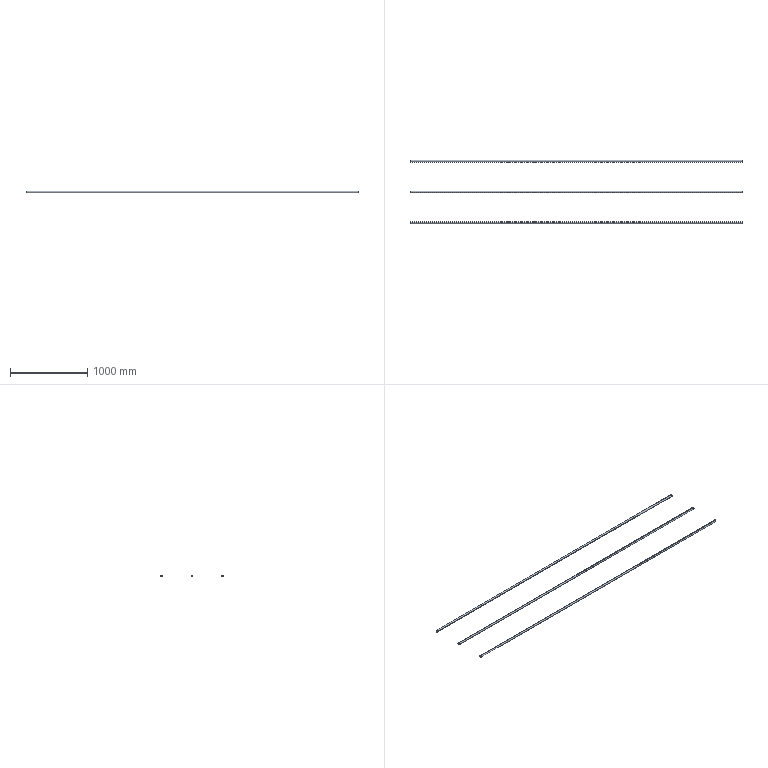Part | STEP file | 电柜护栏4栏杆_Default<As Machined> | 3 solids | 18 faces | box 4293 x 825 x 25 mm | volume 1426235 mm3 | cylinder 12 | plane 6 | commonest cylinder face diameters 22 x6 25 x6
STEP:
#1=CARTESIAN_POINT('',(0.,0.,0.));
#2=DIRECTION('',(0.,0.,1.));
#3=DIRECTION('',(1.,0.,0.));
#4=AXIS2_PLACEMENT_3D('',#1,#2,#3);
#5=CARTESIAN_POINT('',(-4293.,0.,12.5));
#6=VERTEX_POINT('',#5);
#7=CARTESIAN_POINT('',(-4293.,0.,-12.5));
#8=VERTEX_POINT('',#7);
#9=CARTESIAN_POINT('',(-4293.,0.,0.));
#10=DIRECTION('',(-1.,0.,0.));
#11=DIRECTION('',(0.,-1.,0.));
#12=AXIS2_PLACEMENT_3D('',#9,#10,#11);
#13=CIRCLE('',#12,12.5);
#14=CARTESIAN_POINT('',(-4293.,0.,0.));
#15=DIRECTION('',(1.,0.,0.));
#16=DIRECTION('',(0.,0.,-1.));
#17=AXIS2_PLACEMENT_3D('',#14,#15,#16);
#18=CYLINDRICAL_SURFACE('',#17,12.5);
#19=CARTESIAN_POINT('',(4.712,0.));
#20=DIRECTION('',(-1.,0.));
#21=VECTOR('',#20,1.);
#22=LINE('',#19,#21);
#23=(GEOMETRIC_REPRESENTATION_CONTEXT(2)PARAMETRIC_REPRESENTATION_CONTEXT()REPRESENTATION_CONTEXT('',''));
#24=DEFINITIONAL_REPRESENTATION('',(#22),#23);
#25=PCURVE('',#18,#24);
#26=CARTESIAN_POINT('',(-4293.,0.,0.));
#27=DIRECTION('',(-1.,0.,0.));
#28=DIRECTION('',(0.,-1.,0.));
#29=AXIS2_PLACEMENT_3D('',#26,#27,#28);
#30=PLANE('',#29);
#31=CARTESIAN_POINT('',(0.,0.));
#32=DIRECTION('',(1.,0.));
#33=AXIS2_PLACEMENT_2D('',#31,#32);
#34=CIRCLE('',#33,12.5);
#35=(GEOMETRIC_REPRESENTATION_CONTEXT(2)PARAMETRIC_REPRESENTATION_CONTEXT()REPRESENTATION_CONTEXT('',''));
#36=DEFINITIONAL_REPRESENTATION('',(#34),#35);
#37=PCURVE('',#30,#36);
#38=SURFACE_CURVE('',#13,(#25,#37),.PCURVE_S1.);
#39=EDGE_CURVE('',#6,#8,#38,.T.);
#40=ORIENTED_EDGE('',*,*,#39,.F.);
#41=CARTESIAN_POINT('',(0.,0.,12.5));
#42=VERTEX_POINT('',#41);
#43=CARTESIAN_POINT('',(-4293.,0.,12.5));
#44=DIRECTION('',(1.,0.,0.));
#45=VECTOR('',#44,1.);
#46=LINE('',#43,#45);
#47=CARTESIAN_POINT('',(3.142,0.));
#48=DIRECTION('',(0.,1.));
#49=VECTOR('',#48,1.);
#50=LINE('',#47,#49);
#51=(GEOMETRIC_REPRESENTATION_CONTEXT(2)PARAMETRIC_REPRESENTATION_CONTEXT()REPRESENTATION_CONTEXT('',''));
#52=DEFINITIONAL_REPRESENTATION('',(#50),#51);
#53=PCURVE('',#18,#52);
#54=CARTESIAN_POINT('',(-4293.,0.,0.));
#55=DIRECTION('',(1.,0.,0.));
#56=DIRECTION('',(0.,0.,-1.));
#57=AXIS2_PLACEMENT_3D('',#54,#55,#56);
#58=CYLINDRICAL_SURFACE('',#57,12.5);
#59=CARTESIAN_POINT('',(3.142,0.));
#60=DIRECTION('',(0.,1.));
#61=VECTOR('',#60,1.);
#62=LINE('',#59,#61);
#63=(GEOMETRIC_REPRESENTATION_CONTEXT(2)PARAMETRIC_REPRESENTATION_CONTEXT()REPRESENTATION_CONTEXT('',''));
#64=DEFINITIONAL_REPRESENTATION('',(#62),#63);
#65=PCURVE('',#58,#64);
#66=SURFACE_CURVE('',#46,(#53,#65),.PCURVE_S1.);
#67=EDGE_CURVE('',#6,#42,#66,.T.);
#68=ORIENTED_EDGE('',*,*,#67,.T.);
#69=CARTESIAN_POINT('',(0.,0.,-12.5));
#70=VERTEX_POINT('',#69);
#71=CARTESIAN_POINT('',(0.,0.,0.));
#72=DIRECTION('',(-1.,0.,0.));
#73=DIRECTION('',(0.,-1.,0.));
#74=AXIS2_PLACEMENT_3D('',#71,#72,#73);
#75=CIRCLE('',#74,12.5);
#76=CARTESIAN_POINT('',(4.712,4293.));
#77=DIRECTION('',(-1.,0.));
#78=VECTOR('',#77,1.);
#79=LINE('',#76,#78);
#80=(GEOMETRIC_REPRESENTATION_CONTEXT(2)PARAMETRIC_REPRESENTATION_CONTEXT()REPRESENTATION_CONTEXT('',''));
#81=DEFINITIONAL_REPRESENTATION('',(#79),#80);
#82=PCURVE('',#18,#81);
#83=CARTESIAN_POINT('',(0.,0.,0.));
#84=DIRECTION('',(-1.,0.,0.));
#85=DIRECTION('',(0.,-1.,0.));
#86=AXIS2_PLACEMENT_3D('',#83,#84,#85);
#87=PLANE('',#86);
#88=CARTESIAN_POINT('',(0.,0.));
#89=DIRECTION('',(1.,0.));
#90=AXIS2_PLACEMENT_2D('',#88,#89);
#91=CIRCLE('',#90,12.5);
#92=(GEOMETRIC_REPRESENTATION_CONTEXT(2)PARAMETRIC_REPRESENTATION_CONTEXT()REPRESENTATION_CONTEXT('',''));
#93=DEFINITIONAL_REPRESENTATION('',(#91),#92);
#94=PCURVE('',#87,#93);
#95=SURFACE_CURVE('',#75,(#82,#94),.PCURVE_S1.);
#96=EDGE_CURVE('',#42,#70,#95,.T.);
#97=ORIENTED_EDGE('',*,*,#96,.T.);
#98=CARTESIAN_POINT('',(-4293.,0.,-12.5));
#99=DIRECTION('',(1.,0.,0.));
#100=VECTOR('',#99,1.);
#101=LINE('',#98,#100);
#102=CARTESIAN_POINT('',(0.,0.));
#103=DIRECTION('',(0.,1.));
#104=VECTOR('',#103,1.);
#105=LINE('',#102,#104);
#106=(GEOMETRIC_REPRESENTATION_CONTEXT(2)PARAMETRIC_REPRESENTATION_CONTEXT()REPRESENTATION_CONTEXT('',''));
#107=DEFINITIONAL_REPRESENTATION('',(#105),#106);
#108=PCURVE('',#18,#107);
#109=CARTESIAN_POINT('',(6.283,0.));
#110=DIRECTION('',(0.,1.));
#111=VECTOR('',#110,1.);
#112=LINE('',#109,#111);
#113=(GEOMETRIC_REPRESENTATION_CONTEXT(2)PARAMETRIC_REPRESENTATION_CONTEXT()REPRESENTATION_CONTEXT('',''));
#114=DEFINITIONAL_REPRESENTATION('',(#112),#113);
#115=PCURVE('',#58,#114);
#116=SURFACE_CURVE('',#101,(#108,#115),.PCURVE_S1.);
#117=EDGE_CURVE('',#8,#70,#116,.T.);
#118=ORIENTED_EDGE('',*,*,#117,.F.);
#119=EDGE_LOOP('',(#40,#68,#97,#118));
#120=FACE_BOUND('',#119,.T.);
#121=ADVANCED_FACE('',(#120),#18,.T.);
#122=CARTESIAN_POINT('',(-4293.,0.,-11.));
#123=VERTEX_POINT('',#122);
#124=CARTESIAN_POINT('',(0.,0.,-11.));
#125=VERTEX_POINT('',#124);
#126=CARTESIAN_POINT('',(-4293.,0.,-11.));
#127=DIRECTION('',(1.,0.,0.));
#128=VECTOR('',#127,1.);
#129=LINE('',#126,#128);
#130=CARTESIAN_POINT('',(-4293.,0.,0.));
#131=DIRECTION('',(1.,0.,0.));
#132=DIRECTION('',(0.,0.,-1.));
#133=AXIS2_PLACEMENT_3D('',#130,#131,#132);
#134=CYLINDRICAL_SURFACE('',#133,11.);
#135=CARTESIAN_POINT('',(6.283,0.));
#136=DIRECTION('',(0.,1.));
#137=VECTOR('',#136,1.);
#138=LINE('',#135,#137);
#139=(GEOMETRIC_REPRESENTATION_CONTEXT(2)PARAMETRIC_REPRESENTATION_CONTEXT()REPRESENTATION_CONTEXT('',''));
#140=DEFINITIONAL_REPRESENTATION('',(#138),#139);
#141=PCURVE('',#134,#140);
#142=CARTESIAN_POINT('',(-4293.,0.,0.));
#143=DIRECTION('',(1.,0.,0.));
#144=DIRECTION('',(0.,0.,-1.));
#145=AXIS2_PLACEMENT_3D('',#142,#143,#144);
#146=CYLINDRICAL_SURFACE('',#145,11.);
#147=CARTESIAN_POINT('',(0.,0.));
#148=DIRECTION('',(0.,1.));
#149=VECTOR('',#148,1.);
#150=LINE('',#147,#149);
#151=(GEOMETRIC_REPRESENTATION_CONTEXT(2)PARAMETRIC_REPRESENTATION_CONTEXT()REPRESENTATION_CONTEXT('',''));
#152=DEFINITIONAL_REPRESENTATION('',(#150),#151);
#153=PCURVE('',#146,#152);
#154=SURFACE_CURVE('',#129,(#141,#153),.PCURVE_S1.);
#155=EDGE_CURVE('',#123,#125,#154,.T.);
#156=ORIENTED_EDGE('',*,*,#155,.T.);
#157=CARTESIAN_POINT('',(0.,0.,11.));
#158=VERTEX_POINT('',#157);
#159=CARTESIAN_POINT('',(0.,0.,0.));
#160=DIRECTION('',(-1.,0.,0.));
#161=DIRECTION('',(0.,-1.,0.));
#162=AXIS2_PLACEMENT_3D('',#159,#160,#161);
#163=CIRCLE('',#162,11.);
#164=CARTESIAN_POINT('',(10.996,4293.));
#165=DIRECTION('',(-1.,0.));
#166=VECTOR('',#165,1.);
#167=LINE('',#164,#166);
#168=(GEOMETRIC_REPRESENTATION_CONTEXT(2)PARAMETRIC_REPRESENTATION_CONTEXT()REPRESENTATION_CONTEXT('',''));
#169=DEFINITIONAL_REPRESENTATION('',(#167),#168);
#170=PCURVE('',#134,#169);
#171=CARTESIAN_POINT('',(0.,0.));
#172=DIRECTION('',(1.,0.));
#173=AXIS2_PLACEMENT_2D('',#171,#172);
#174=CIRCLE('',#173,11.);
#175=(GEOMETRIC_REPRESENTATION_CONTEXT(2)PARAMETRIC_REPRESENTATION_CONTEXT()REPRESENTATION_CONTEXT('',''));
#176=DEFINITIONAL_REPRESENTATION('',(#174),#175);
#177=PCURVE('',#87,#176);
#178=SURFACE_CURVE('',#163,(#170,#177),.PCURVE_S1.);
#179=EDGE_CURVE('',#125,#158,#178,.T.);
#180=ORIENTED_EDGE('',*,*,#179,.T.);
#181=CARTESIAN_POINT('',(-4293.,0.,11.));
#182=VERTEX_POINT('',#181);
#183=CARTESIAN_POINT('',(-4293.,0.,11.));
#184=DIRECTION('',(1.,0.,0.));
#185=VECTOR('',#184,1.);
#186=LINE('',#183,#185);
#187=CARTESIAN_POINT('',(3.142,0.));
#188=DIRECTION('',(0.,1.));
#189=VECTOR('',#188,1.);
#190=LINE('',#187,#189);
#191=(GEOMETRIC_REPRESENTATION_CONTEXT(2)PARAMETRIC_REPRESENTATION_CONTEXT()REPRESENTATION_CONTEXT('',''));
#192=DEFINITIONAL_REPRESENTATION('',(#190),#191);
#193=PCURVE('',#134,#192);
#194=CARTESIAN_POINT('',(3.142,0.));
#195=DIRECTION('',(0.,1.));
#196=VECTOR('',#195,1.);
#197=LINE('',#194,#196);
#198=(GEOMETRIC_REPRESENTATION_CONTEXT(2)PARAMETRIC_REPRESENTATION_CONTEXT()REPRESENTATION_CONTEXT('',''));
#199=DEFINITIONAL_REPRESENTATION('',(#197),#198);
#200=PCURVE('',#146,#199);
#201=SURFACE_CURVE('',#186,(#193,#200),.PCURVE_S1.);
#202=EDGE_CURVE('',#182,#158,#201,.T.);
#203=ORIENTED_EDGE('',*,*,#202,.F.);
#204=CARTESIAN_POINT('',(-4293.,0.,0.));
#205=DIRECTION('',(-1.,0.,0.));
#206=DIRECTION('',(0.,-1.,0.));
#207=AXIS2_PLACEMENT_3D('',#204,#205,#206);
#208=CIRCLE('',#207,11.);
#209=CARTESIAN_POINT('',(10.996,0.));
#210=DIRECTION('',(-1.,0.));
#211=VECTOR('',#210,1.);
#212=LINE('',#209,#211);
#213=(GEOMETRIC_REPRESENTATION_CONTEXT(2)PARAMETRIC_REPRESENTATION_CONTEXT()REPRESENTATION_CONTEXT('',''));
#214=DEFINITIONAL_REPRESENTATION('',(#212),#213);
#215=PCURVE('',#134,#214);
#216=CARTESIAN_POINT('',(0.,0.));
#217=DIRECTION('',(1.,0.));
#218=AXIS2_PLACEMENT_2D('',#216,#217);
#219=CIRCLE('',#218,11.);
#220=(GEOMETRIC_REPRESENTATION_CONTEXT(2)PARAMETRIC_REPRESENTATION_CONTEXT()REPRESENTATION_CONTEXT('',''));
#221=DEFINITIONAL_REPRESENTATION('',(#219),#220);
#222=PCURVE('',#30,#221);
#223=SURFACE_CURVE('',#208,(#215,#222),.PCURVE_S1.);
#224=EDGE_CURVE('',#123,#182,#223,.T.);
#225=ORIENTED_EDGE('',*,*,#224,.F.);
#226=EDGE_LOOP('',(#156,#180,#203,#225));
#227=FACE_BOUND('',#226,.F.);
#228=ADVANCED_FACE('',(#227),#134,.F.);
#229=CARTESIAN_POINT('',(0.,0.,0.));
#230=DIRECTION('',(-1.,0.,0.));
#231=DIRECTION('',(0.,-1.,0.));
#232=AXIS2_PLACEMENT_3D('',#229,#230,#231);
#233=CIRCLE('',#232,11.);
#234=CARTESIAN_POINT('',(4.712,4293.));
#235=DIRECTION('',(-1.,0.));
#236=VECTOR('',#235,1.);
#237=LINE('',#234,#236);
#238=(GEOMETRIC_REPRESENTATION_CONTEXT(2)PARAMETRIC_REPRESENTATION_CONTEXT()REPRESENTATION_CONTEXT('',''));
#239=DEFINITIONAL_REPRESENTATION('',(#237),#238);
#240=PCURVE('',#146,#239);
#241=CARTESIAN_POINT('',(0.,0.));
#242=DIRECTION('',(1.,0.));
#243=AXIS2_PLACEMENT_2D('',#241,#242);
#244=CIRCLE('',#243,11.);
#245=(GEOMETRIC_REPRESENTATION_CONTEXT(2)PARAMETRIC_REPRESENTATION_CONTEXT()REPRESENTATION_CONTEXT('',''));
#246=DEFINITIONAL_REPRESENTATION('',(#244),#245);
#247=PCURVE('',#87,#246);
#248=SURFACE_CURVE('',#233,(#240,#247),.PCURVE_S1.);
#249=EDGE_CURVE('',#158,#125,#248,.T.);
#250=ORIENTED_EDGE('',*,*,#249,.T.);
#251=ORIENTED_EDGE('',*,*,#155,.F.);
#252=CARTESIAN_POINT('',(-4293.,0.,0.));
#253=DIRECTION('',(-1.,0.,0.));
#254=DIRECTION('',(0.,-1.,0.));
#255=AXIS2_PLACEMENT_3D('',#252,#253,#254);
#256=CIRCLE('',#255,11.);
#257=CARTESIAN_POINT('',(4.712,0.));
#258=DIRECTION('',(-1.,0.));
#259=VECTOR('',#258,1.);
#260=LINE('',#257,#259);
#261=(GEOMETRIC_REPRESENTATION_CONTEXT(2)PARAMETRIC_REPRESENTATION_CONTEXT()REPRESENTATION_CONTEXT('',''));
#262=DEFINITIONAL_REPRESENTATION('',(#260),#261);
#263=PCURVE('',#146,#262);
#264=CARTESIAN_POINT('',(0.,0.));
#265=DIRECTION('',(1.,0.));
#266=AXIS2_PLACEMENT_2D('',#264,#265);
#267=CIRCLE('',#266,11.);
#268=(GEOMETRIC_REPRESENTATION_CONTEXT(2)PARAMETRIC_REPRESENTATION_CONTEXT()REPRESENTATION_CONTEXT('',''));
#269=DEFINITIONAL_REPRESENTATION('',(#267),#268);
#270=PCURVE('',#30,#269);
#271=SURFACE_CURVE('',#256,(#263,#270),.PCURVE_S1.);
#272=EDGE_CURVE('',#182,#123,#271,.T.);
#273=ORIENTED_EDGE('',*,*,#272,.F.);
#274=ORIENTED_EDGE('',*,*,#202,.T.);
#275=EDGE_LOOP('',(#250,#251,#273,#274));
#276=FACE_BOUND('',#275,.F.);
#277=ADVANCED_FACE('',(#276),#146,.F.);
#278=ORIENTED_EDGE('',*,*,#67,.F.);
#279=CARTESIAN_POINT('',(-4293.,0.,0.));
#280=DIRECTION('',(-1.,0.,0.));
#281=DIRECTION('',(0.,-1.,0.));
#282=AXIS2_PLACEMENT_3D('',#279,#280,#281);
#283=CIRCLE('',#282,12.5);
#284=CARTESIAN_POINT('',(10.996,0.));
#285=DIRECTION('',(-1.,0.));
#286=VECTOR('',#285,1.);
#287=LINE('',#284,#286);
#288=(GEOMETRIC_REPRESENTATION_CONTEXT(2)PARAMETRIC_REPRESENTATION_CONTEXT()REPRESENTATION_CONTEXT('',''));
#289=DEFINITIONAL_REPRESENTATION('',(#287),#288);
#290=PCURVE('',#58,#289);
#291=CARTESIAN_POINT('',(0.,0.));
#292=DIRECTION('',(1.,0.));
#293=AXIS2_PLACEMENT_2D('',#291,#292);
#294=CIRCLE('',#293,12.5);
#295=(GEOMETRIC_REPRESENTATION_CONTEXT(2)PARAMETRIC_REPRESENTATION_CONTEXT()REPRESENTATION_CONTEXT('',''));
#296=DEFINITIONAL_REPRESENTATION('',(#294),#295);
#297=PCURVE('',#30,#296);
#298=SURFACE_CURVE('',#283,(#290,#297),.PCURVE_S1.);
#299=EDGE_CURVE('',#8,#6,#298,.T.);
#300=ORIENTED_EDGE('',*,*,#299,.F.);
#301=ORIENTED_EDGE('',*,*,#117,.T.);
#302=CARTESIAN_POINT('',(0.,0.,0.));
#303=DIRECTION('',(-1.,0.,0.));
#304=DIRECTION('',(0.,-1.,0.));
#305=AXIS2_PLACEMENT_3D('',#302,#303,#304);
#306=CIRCLE('',#305,12.5);
#307=CARTESIAN_POINT('',(10.996,4293.));
#308=DIRECTION('',(-1.,0.));
#309=VECTOR('',#308,1.);
#310=LINE('',#307,#309);
#311=(GEOMETRIC_REPRESENTATION_CONTEXT(2)PARAMETRIC_REPRESENTATION_CONTEXT()REPRESENTATION_CONTEXT('',''));
#312=DEFINITIONAL_REPRESENTATION('',(#310),#311);
#313=PCURVE('',#58,#312);
#314=CARTESIAN_POINT('',(0.,0.));
#315=DIRECTION('',(1.,0.));
#316=AXIS2_PLACEMENT_2D('',#314,#315);
#317=CIRCLE('',#316,12.5);
#318=(GEOMETRIC_REPRESENTATION_CONTEXT(2)PARAMETRIC_REPRESENTATION_CONTEXT()REPRESENTATION_CONTEXT('',''));
#319=DEFINITIONAL_REPRESENTATION('',(#317),#318);
#320=PCURVE('',#87,#319);
#321=SURFACE_CURVE('',#306,(#313,#320),.PCURVE_S1.);
#322=EDGE_CURVE('',#70,#42,#321,.T.);
#323=ORIENTED_EDGE('',*,*,#322,.T.);
#324=EDGE_LOOP('',(#278,#300,#301,#323));
#325=FACE_BOUND('',#324,.T.);
#326=ADVANCED_FACE('',(#325),#58,.T.);
#327=ORIENTED_EDGE('',*,*,#224,.F.);
#328=ORIENTED_EDGE('',*,*,#272,.F.);
#329=EDGE_LOOP('',(#327,#328));
#330=FACE_BOUND('',#329,.T.);
#331=ORIENTED_EDGE('',*,*,#299,.T.);
#332=ORIENTED_EDGE('',*,*,#39,.T.);
#333=EDGE_LOOP('',(#331,#332));
#334=FACE_BOUND('',#333,.T.);
#335=ADVANCED_FACE('',(#330,#334),#30,.T.);
#336=ORIENTED_EDGE('',*,*,#179,.T.);
#337=ORIENTED_EDGE('',*,*,#249,.T.);
#338=EDGE_LOOP('',(#336,#337));
#339=FACE_BOUND('',#338,.T.);
#340=ORIENTED_EDGE('',*,*,#322,.F.);
#341=ORIENTED_EDGE('',*,*,#96,.F.);
#342=EDGE_LOOP('',(#340,#341));
#343=FACE_BOUND('',#342,.T.);
#344=ADVANCED_FACE('',(#339,#343),#87,.F.);
#345=CLOSED_SHELL('',(#121,#228,#277,#326,#335,#344));
#346=MANIFOLD_SOLID_BREP('',#345);
#347=CARTESIAN_POINT('',(-4293.,787.5,0.));
#348=VERTEX_POINT('',#347);
#349=CARTESIAN_POINT('',(-4293.,812.5,0.));
#350=VERTEX_POINT('',#349);
#351=CARTESIAN_POINT('',(-4293.,800.,0.));
#352=DIRECTION('',(-1.,0.,0.));
#353=DIRECTION('',(0.,-1.,0.));
#354=AXIS2_PLACEMENT_3D('',#351,#352,#353);
#355=CIRCLE('',#354,12.5);
#356=CARTESIAN_POINT('',(-4293.,800.,0.));
#357=DIRECTION('',(1.,0.,0.));
#358=DIRECTION('',(0.,1.,0.));
#359=AXIS2_PLACEMENT_3D('',#356,#357,#358);
#360=CYLINDRICAL_SURFACE('',#359,12.5);
#361=CARTESIAN_POINT('',(3.142,0.));
#362=DIRECTION('',(-1.,0.));
#363=VECTOR('',#362,1.);
#364=LINE('',#361,#363);
#365=(GEOMETRIC_REPRESENTATION_CONTEXT(2)PARAMETRIC_REPRESENTATION_CONTEXT()REPRESENTATION_CONTEXT('',''));
#366=DEFINITIONAL_REPRESENTATION('',(#364),#365);
#367=PCURVE('',#360,#366);
#368=CARTESIAN_POINT('',(-4293.,800.,0.));
#369=DIRECTION('',(-1.,0.,0.));
#370=DIRECTION('',(0.,-1.,0.));
#371=AXIS2_PLACEMENT_3D('',#368,#369,#370);
#372=PLANE('',#371);
#373=CARTESIAN_POINT('',(0.,0.));
#374=DIRECTION('',(1.,0.));
#375=AXIS2_PLACEMENT_2D('',#373,#374);
#376=CIRCLE('',#375,12.5);
#377=(GEOMETRIC_REPRESENTATION_CONTEXT(2)PARAMETRIC_REPRESENTATION_CONTEXT()REPRESENTATION_CONTEXT('',''));
#378=DEFINITIONAL_REPRESENTATION('',(#376),#377);
#379=PCURVE('',#372,#378);
#380=SURFACE_CURVE('',#355,(#367,#379),.PCURVE_S1.);
#381=EDGE_CURVE('',#348,#350,#380,.T.);
#382=ORIENTED_EDGE('',*,*,#381,.F.);
#383=CARTESIAN_POINT('',(0.,787.5,0.));
#384=VERTEX_POINT('',#383);
#385=CARTESIAN_POINT('',(-4293.,787.5,0.));
#386=DIRECTION('',(1.,0.,0.));
#387=VECTOR('',#386,1.);
#388=LINE('',#385,#387);
#389=CARTESIAN_POINT('',(3.142,0.));
#390=DIRECTION('',(0.,1.));
#391=VECTOR('',#390,1.);
#392=LINE('',#389,#391);
#393=(GEOMETRIC_REPRESENTATION_CONTEXT(2)PARAMETRIC_REPRESENTATION_CONTEXT()REPRESENTATION_CONTEXT('',''));
#394=DEFINITIONAL_REPRESENTATION('',(#392),#393);
#395=PCURVE('',#360,#394);
#396=CARTESIAN_POINT('',(-4293.,800.,0.));
#397=DIRECTION('',(1.,0.,0.));
#398=DIRECTION('',(0.,1.,0.));
#399=AXIS2_PLACEMENT_3D('',#396,#397,#398);
#400=CYLINDRICAL_SURFACE('',#399,12.5);
#401=CARTESIAN_POINT('',(3.142,0.));
#402=DIRECTION('',(0.,1.));
#403=VECTOR('',#402,1.);
#404=LINE('',#401,#403);
#405=(GEOMETRIC_REPRESENTATION_CONTEXT(2)PARAMETRIC_REPRESENTATION_CONTEXT()REPRESENTATION_CONTEXT('',''));
#406=DEFINITIONAL_REPRESENTATION('',(#404),#405);
#407=PCURVE('',#400,#406);
#408=SURFACE_CURVE('',#388,(#395,#407),.PCURVE_S1.);
#409=EDGE_CURVE('',#348,#384,#408,.T.);
#410=ORIENTED_EDGE('',*,*,#409,.T.);
#411=CARTESIAN_POINT('',(0.,812.5,0.));
#412=VERTEX_POINT('',#411);
#413=CARTESIAN_POINT('',(0.,800.,0.));
#414=DIRECTION('',(-1.,0.,0.));
#415=DIRECTION('',(0.,-1.,0.));
#416=AXIS2_PLACEMENT_3D('',#413,#414,#415);
#417=CIRCLE('',#416,12.5);
#418=CARTESIAN_POINT('',(3.142,4293.));
#419=DIRECTION('',(-1.,0.));
#420=VECTOR('',#419,1.);
#421=LINE('',#418,#420);
#422=(GEOMETRIC_REPRESENTATION_CONTEXT(2)PARAMETRIC_REPRESENTATION_CONTEXT()REPRESENTATION_CONTEXT('',''));
#423=DEFINITIONAL_REPRESENTATION('',(#421),#422);
#424=PCURVE('',#360,#423);
#425=CARTESIAN_POINT('',(0.,800.,0.));
#426=DIRECTION('',(-1.,0.,0.));
#427=DIRECTION('',(0.,-1.,0.));
#428=AXIS2_PLACEMENT_3D('',#425,#426,#427);
#429=PLANE('',#428);
#430=CARTESIAN_POINT('',(0.,0.));
#431=DIRECTION('',(1.,0.));
#432=AXIS2_PLACEMENT_2D('',#430,#431);
#433=CIRCLE('',#432,12.5);
#434=(GEOMETRIC_REPRESENTATION_CONTEXT(2)PARAMETRIC_REPRESENTATION_CONTEXT()REPRESENTATION_CONTEXT('',''));
#435=DEFINITIONAL_REPRESENTATION('',(#433),#434);
#436=PCURVE('',#429,#435);
#437=SURFACE_CURVE('',#417,(#424,#436),.PCURVE_S1.);
#438=EDGE_CURVE('',#384,#412,#437,.T.);
#439=ORIENTED_EDGE('',*,*,#438,.T.);
#440=CARTESIAN_POINT('',(-4293.,812.5,0.));
#441=DIRECTION('',(1.,0.,0.));
#442=VECTOR('',#441,1.);
#443=LINE('',#440,#442);
#444=CARTESIAN_POINT('',(0.,0.));
#445=DIRECTION('',(0.,1.));
#446=VECTOR('',#445,1.);
#447=LINE('',#444,#446);
#448=(GEOMETRIC_REPRESENTATION_CONTEXT(2)PARAMETRIC_REPRESENTATION_CONTEXT()REPRESENTATION_CONTEXT('',''));
#449=DEFINITIONAL_REPRESENTATION('',(#447),#448);
#450=PCURVE('',#360,#449);
#451=CARTESIAN_POINT('',(6.283,0.));
#452=DIRECTION('',(0.,1.));
#453=VECTOR('',#452,1.);
#454=LINE('',#451,#453);
#455=(GEOMETRIC_REPRESENTATION_CONTEXT(2)PARAMETRIC_REPRESENTATION_CONTEXT()REPRESENTATION_CONTEXT('',''));
#456=DEFINITIONAL_REPRESENTATION('',(#454),#455);
#457=PCURVE('',#400,#456);
#458=SURFACE_CURVE('',#443,(#450,#457),.PCURVE_S1.);
#459=EDGE_CURVE('',#350,#412,#458,.T.);
#460=ORIENTED_EDGE('',*,*,#459,.F.);
#461=EDGE_LOOP('',(#382,#410,#439,#460));
#462=FACE_BOUND('',#461,.T.);
#463=ADVANCED_FACE('',(#462),#360,.T.);
#464=CARTESIAN_POINT('',(-4293.,811.,0.));
#465=VERTEX_POINT('',#464);
#466=CARTESIAN_POINT('',(0.,811.,0.));
#467=VERTEX_POINT('',#466);
#468=CARTESIAN_POINT('',(-4293.,811.,0.));
#469=DIRECTION('',(1.,0.,0.));
#470=VECTOR('',#469,1.);
#471=LINE('',#468,#470);
#472=CARTESIAN_POINT('',(-4293.,800.,0.));
#473=DIRECTION('',(1.,0.,0.));
#474=DIRECTION('',(0.,1.,0.));
#475=AXIS2_PLACEMENT_3D('',#472,#473,#474);
#476=CYLINDRICAL_SURFACE('',#475,11.);
#477=CARTESIAN_POINT('',(6.283,0.));
#478=DIRECTION('',(0.,1.));
#479=VECTOR('',#478,1.);
#480=LINE('',#477,#479);
#481=(GEOMETRIC_REPRESENTATION_CONTEXT(2)PARAMETRIC_REPRESENTATION_CONTEXT()REPRESENTATION_CONTEXT('',''));
#482=DEFINITIONAL_REPRESENTATION('',(#480),#481);
#483=PCURVE('',#476,#482);
#484=CARTESIAN_POINT('',(-4293.,800.,0.));
#485=DIRECTION('',(1.,0.,0.));
#486=DIRECTION('',(0.,1.,0.));
#487=AXIS2_PLACEMENT_3D('',#484,#485,#486);
#488=CYLINDRICAL_SURFACE('',#487,11.);
#489=CARTESIAN_POINT('',(0.,0.));
#490=DIRECTION('',(0.,1.));
#491=VECTOR('',#490,1.);
#492=LINE('',#489,#491);
#493=(GEOMETRIC_REPRESENTATION_CONTEXT(2)PARAMETRIC_REPRESENTATION_CONTEXT()REPRESENTATION_CONTEXT('',''));
#494=DEFINITIONAL_REPRESENTATION('',(#492),#493);
#495=PCURVE('',#488,#494);
#496=SURFACE_CURVE('',#471,(#483,#495),.PCURVE_S1.);
#497=EDGE_CURVE('',#465,#467,#496,.T.);
#498=ORIENTED_EDGE('',*,*,#497,.T.);
#499=CARTESIAN_POINT('',(0.,789.,0.));
#500=VERTEX_POINT('',#499);
#501=CARTESIAN_POINT('',(0.,800.,0.));
#502=DIRECTION('',(-1.,0.,0.));
#503=DIRECTION('',(0.,-1.,0.));
#504=AXIS2_PLACEMENT_3D('',#501,#502,#503);
#505=CIRCLE('',#504,11.);
#506=CARTESIAN_POINT('',(9.425,4293.));
#507=DIRECTION('',(-1.,0.));
#508=VECTOR('',#507,1.);
#509=LINE('',#506,#508);
#510=(GEOMETRIC_REPRESENTATION_CONTEXT(2)PARAMETRIC_REPRESENTATION_CONTEXT()REPRESENTATION_CONTEXT('',''));
#511=DEFINITIONAL_REPRESENTATION('',(#509),#510);
#512=PCURVE('',#476,#511);
#513=CARTESIAN_POINT('',(0.,0.));
#514=DIRECTION('',(1.,0.));
#515=AXIS2_PLACEMENT_2D('',#513,#514);
#516=CIRCLE('',#515,11.);
#517=(GEOMETRIC_REPRESENTATION_CONTEXT(2)PARAMETRIC_REPRESENTATION_CONTEXT()REPRESENTATION_CONTEXT('',''));
#518=DEFINITIONAL_REPRESENTATION('',(#516),#517);
#519=PCURVE('',#429,#518);
#520=SURFACE_CURVE('',#505,(#512,#519),.PCURVE_S1.);
#521=EDGE_CURVE('',#467,#500,#520,.T.);
#522=ORIENTED_EDGE('',*,*,#521,.T.);
#523=CARTESIAN_POINT('',(-4293.,789.,0.));
#524=VERTEX_POINT('',#523);
#525=CARTESIAN_POINT('',(-4293.,789.,0.));
#526=DIRECTION('',(1.,0.,0.));
#527=VECTOR('',#526,1.);
#528=LINE('',#525,#527);
#529=CARTESIAN_POINT('',(3.142,0.));
#530=DIRECTION('',(0.,1.));
#531=VECTOR('',#530,1.);
#532=LINE('',#529,#531);
#533=(GEOMETRIC_REPRESENTATION_CONTEXT(2)PARAMETRIC_REPRESENTATION_CONTEXT()REPRESENTATION_CONTEXT('',''));
#534=DEFINITIONAL_REPRESENTATION('',(#532),#533);
#535=PCURVE('',#476,#534);
#536=CARTESIAN_POINT('',(3.142,0.));
#537=DIRECTION('',(0.,1.));
#538=VECTOR('',#537,1.);
#539=LINE('',#536,#538);
#540=(GEOMETRIC_REPRESENTATION_CONTEXT(2)PARAMETRIC_REPRESENTATION_CONTEXT()REPRESENTATION_CONTEXT('',''));
#541=DEFINITIONAL_REPRESENTATION('',(#539),#540);
#542=PCURVE('',#488,#541);
#543=SURFACE_CURVE('',#528,(#535,#542),.PCURVE_S1.);
#544=EDGE_CURVE('',#524,#500,#543,.T.);
#545=ORIENTED_EDGE('',*,*,#544,.F.);
#546=CARTESIAN_POINT('',(-4293.,800.,0.));
#547=DIRECTION('',(-1.,0.,0.));
#548=DIRECTION('',(0.,-1.,0.));
#549=AXIS2_PLACEMENT_3D('',#546,#547,#548);
#550=CIRCLE('',#549,11.);
#551=CARTESIAN_POINT('',(9.425,0.));
#552=DIRECTION('',(-1.,0.));
#553=VECTOR('',#552,1.);
#554=LINE('',#551,#553);
#555=(GEOMETRIC_REPRESENTATION_CONTEXT(2)PARAMETRIC_REPRESENTATION_CONTEXT()REPRESENTATION_CONTEXT('',''));
#556=DEFINITIONAL_REPRESENTATION('',(#554),#555);
#557=PCURVE('',#476,#556);
#558=CARTESIAN_POINT('',(0.,0.));
#559=DIRECTION('',(1.,0.));
#560=AXIS2_PLACEMENT_2D('',#558,#559);
#561=CIRCLE('',#560,11.);
#562=(GEOMETRIC_REPRESENTATION_CONTEXT(2)PARAMETRIC_REPRESENTATION_CONTEXT()REPRESENTATION_CONTEXT('',''));
#563=DEFINITIONAL_REPRESENTATION('',(#561),#562);
#564=PCURVE('',#372,#563);
#565=SURFACE_CURVE('',#550,(#557,#564),.PCURVE_S1.);
#566=EDGE_CURVE('',#465,#524,#565,.T.);
#567=ORIENTED_EDGE('',*,*,#566,.F.);
#568=EDGE_LOOP('',(#498,#522,#545,#567));
#569=FACE_BOUND('',#568,.F.);
#570=ADVANCED_FACE('',(#569),#476,.F.);
#571=CARTESIAN_POINT('',(0.,800.,0.));
#572=DIRECTION('',(-1.,0.,0.));
#573=DIRECTION('',(0.,-1.,0.));
#574=AXIS2_PLACEMENT_3D('',#571,#572,#573);
#575=CIRCLE('',#574,11.);
#576=CARTESIAN_POINT('',(3.142,4293.));
#577=DIRECTION('',(-1.,0.));
#578=VECTOR('',#577,1.);
#579=LINE('',#576,#578);
#580=(GEOMETRIC_REPRESENTATION_CONTEXT(2)PARAMETRIC_REPRESENTATION_CONTEXT()REPRESENTATION_CONTEXT('',''));
#581=DEFINITIONAL_REPRESENTATION('',(#579),#580);
#582=PCURVE('',#488,#581);
#583=CARTESIAN_POINT('',(0.,0.));
#584=DIRECTION('',(1.,0.));
#585=AXIS2_PLACEMENT_2D('',#583,#584);
#586=CIRCLE('',#585,11.);
#587=(GEOMETRIC_REPRESENTATION_CONTEXT(2)PARAMETRIC_REPRESENTATION_CONTEXT()REPRESENTATION_CONTEXT('',''));
#588=DEFINITIONAL_REPRESENTATION('',(#586),#587);
#589=PCURVE('',#429,#588);
#590=SURFACE_CURVE('',#575,(#582,#589),.PCURVE_S1.);
#591=EDGE_CURVE('',#500,#467,#590,.T.);
#592=ORIENTED_EDGE('',*,*,#591,.T.);
#593=ORIENTED_EDGE('',*,*,#497,.F.);
#594=CARTESIAN_POINT('',(-4293.,800.,0.));
#595=DIRECTION('',(-1.,0.,0.));
#596=DIRECTION('',(0.,-1.,0.));
#597=AXIS2_PLACEMENT_3D('',#594,#595,#596);
#598=CIRCLE('',#597,11.);
#599=CARTESIAN_POINT('',(3.142,0.));
#600=DIRECTION('',(-1.,0.));
#601=VECTOR('',#600,1.);
#602=LINE('',#599,#601);
#603=(GEOMETRIC_REPRESENTATION_CONTEXT(2)PARAMETRIC_REPRESENTATION_CONTEXT()REPRESENTATION_CONTEXT('',''));
#604=DEFINITIONAL_REPRESENTATION('',(#602),#603);
#605=PCURVE('',#488,#604);
#606=CARTESIAN_POINT('',(0.,0.));
#607=DIRECTION('',(1.,0.));
#608=AXIS2_PLACEMENT_2D('',#606,#607);
#609=CIRCLE('',#608,11.);
#610=(GEOMETRIC_REPRESENTATION_CONTEXT(2)PARAMETRIC_REPRESENTATION_CONTEXT()REPRESENTATION_CONTEXT('',''));
#611=DEFINITIONAL_REPRESENTATION('',(#609),#610);
#612=PCURVE('',#372,#611);
#613=SURFACE_CURVE('',#598,(#605,#612),.PCURVE_S1.);
#614=EDGE_CURVE('',#524,#465,#613,.T.);
#615=ORIENTED_EDGE('',*,*,#614,.F.);
#616=ORIENTED_EDGE('',*,*,#544,.T.);
#617=EDGE_LOOP('',(#592,#593,#615,#616));
#618=FACE_BOUND('',#617,.F.);
#619=ADVANCED_FACE('',(#618),#488,.F.);
#620=ORIENTED_EDGE('',*,*,#409,.F.);
#621=CARTESIAN_POINT('',(-4293.,800.,0.));
#622=DIRECTION('',(-1.,0.,0.));
#623=DIRECTION('',(0.,-1.,0.));
#624=AXIS2_PLACEMENT_3D('',#621,#622,#623);
#625=CIRCLE('',#624,12.5);
#626=CARTESIAN_POINT('',(9.425,0.));
#627=DIRECTION('',(-1.,0.));
#628=VECTOR('',#627,1.);
#629=LINE('',#626,#628);
#630=(GEOMETRIC_REPRESENTATION_CONTEXT(2)PARAMETRIC_REPRESENTATION_CONTEXT()REPRESENTATION_CONTEXT('',''));
#631=DEFINITIONAL_REPRESENTATION('',(#629),#630);
#632=PCURVE('',#400,#631);
#633=CARTESIAN_POINT('',(0.,0.));
#634=DIRECTION('',(1.,0.));
#635=AXIS2_PLACEMENT_2D('',#633,#634);
#636=CIRCLE('',#635,12.5);
#637=(GEOMETRIC_REPRESENTATION_CONTEXT(2)PARAMETRIC_REPRESENTATION_CONTEXT()REPRESENTATION_CONTEXT('',''));
#638=DEFINITIONAL_REPRESENTATION('',(#636),#637);
#639=PCURVE('',#372,#638);
#640=SURFACE_CURVE('',#625,(#632,#639),.PCURVE_S1.);
#641=EDGE_CURVE('',#350,#348,#640,.T.);
#642=ORIENTED_EDGE('',*,*,#641,.F.);
#643=ORIENTED_EDGE('',*,*,#459,.T.);
#644=CARTESIAN_POINT('',(0.,800.,0.));
#645=DIRECTION('',(-1.,0.,0.));
#646=DIRECTION('',(0.,-1.,0.));
#647=AXIS2_PLACEMENT_3D('',#644,#645,#646);
#648=CIRCLE('',#647,12.5);
#649=CARTESIAN_POINT('',(9.425,4293.));
#650=DIRECTION('',(-1.,0.));
#651=VECTOR('',#650,1.);
#652=LINE('',#649,#651);
#653=(GEOMETRIC_REPRESENTATION_CONTEXT(2)PARAMETRIC_REPRESENTATION_CONTEXT()REPRESENTATION_CONTEXT('',''));
#654=DEFINITIONAL_REPRESENTATION('',(#652),#653);
#655=PCURVE('',#400,#654);
#656=CARTESIAN_POINT('',(0.,0.));
#657=DIRECTION('',(1.,0.));
#658=AXIS2_PLACEMENT_2D('',#656,#657);
#659=CIRCLE('',#658,12.5);
#660=(GEOMETRIC_REPRESENTATION_CONTEXT(2)PARAMETRIC_REPRESENTATION_CONTEXT()REPRESENTATION_CONTEXT('',''));
#661=DEFINITIONAL_REPRESENTATION('',(#659),#660);
#662=PCURVE('',#429,#661);
#663=SURFACE_CURVE('',#648,(#655,#662),.PCURVE_S1.);
#664=EDGE_CURVE('',#412,#384,#663,.T.);
#665=ORIENTED_EDGE('',*,*,#664,.T.);
#666=EDGE_LOOP('',(#620,#642,#643,#665));
#667=FACE_BOUND('',#666,.T.);
#668=ADVANCED_FACE('',(#667),#400,.T.);
#669=ORIENTED_EDGE('',*,*,#566,.F.);
#670=ORIENTED_EDGE('',*,*,#614,.F.);
#671=EDGE_LOOP('',(#669,#670));
#672=FACE_BOUND('',#671,.T.);
#673=ORIENTED_EDGE('',*,*,#641,.T.);
#674=ORIENTED_EDGE('',*,*,#381,.T.);
#675=EDGE_LOOP('',(#673,#674));
#676=FACE_BOUND('',#675,.T.);
#677=ADVANCED_FACE('',(#672,#676),#372,.T.);
#678=ORIENTED_EDGE('',*,*,#521,.T.);
#679=ORIENTED_EDGE('',*,*,#591,.T.);
#680=EDGE_LOOP('',(#678,#679));
#681=FACE_BOUND('',#680,.T.);
#682=ORIENTED_EDGE('',*,*,#664,.F.);
#683=ORIENTED_EDGE('',*,*,#438,.F.);
#684=EDGE_LOOP('',(#682,#683));
#685=FACE_BOUND('',#684,.T.);
#686=ADVANCED_FACE('',(#681,#685),#429,.F.);
#687=CLOSED_SHELL('',(#463,#570,#619,#668,#677,#686));
#688=MANIFOLD_SOLID_BREP('',#687);
#689=CARTESIAN_POINT('',(0.,400.,-12.5));
#690=VERTEX_POINT('',#689);
#691=CARTESIAN_POINT('',(0.,400.,12.5));
#692=VERTEX_POINT('',#691);
#693=CARTESIAN_POINT('',(0.,400.,0.));
#694=DIRECTION('',(1.,0.,0.));
#695=DIRECTION('',(0.,1.,0.));
#696=AXIS2_PLACEMENT_3D('',#693,#694,#695);
#697=CIRCLE('',#696,12.5);
#698=CARTESIAN_POINT('',(0.,400.,0.));
#699=DIRECTION('',(-1.,0.,0.));
#700=DIRECTION('',(0.,0.,1.));
#701=AXIS2_PLACEMENT_3D('',#698,#699,#700);
#702=CYLINDRICAL_SURFACE('',#701,12.5);
#703=CARTESIAN_POINT('',(7.854,0.));
#704=DIRECTION('',(-1.,0.));
#705=VECTOR('',#704,1.);
#706=LINE('',#703,#705);
#707=(GEOMETRIC_REPRESENTATION_CONTEXT(2)PARAMETRIC_REPRESENTATION_CONTEXT()REPRESENTATION_CONTEXT('',''));
#708=DEFINITIONAL_REPRESENTATION('',(#706),#707);
#709=PCURVE('',#702,#708);
#710=CARTESIAN_POINT('',(0.,400.,0.));
#711=DIRECTION('',(1.,0.,0.));
#712=DIRECTION('',(0.,1.,0.));
#713=AXIS2_PLACEMENT_3D('',#710,#711,#712);
#714=PLANE('',#713);
#715=CARTESIAN_POINT('',(0.,0.));
#716=DIRECTION('',(1.,0.));
#717=AXIS2_PLACEMENT_2D('',#715,#716);
#718=CIRCLE('',#717,12.5);
#719=(GEOMETRIC_REPRESENTATION_CONTEXT(2)PARAMETRIC_REPRESENTATION_CONTEXT()REPRESENTATION_CONTEXT('',''));
#720=DEFINITIONAL_REPRESENTATION('',(#718),#719);
#721=PCURVE('',#714,#720);
#722=SURFACE_CURVE('',#697,(#709,#721),.PCURVE_S1.);
#723=EDGE_CURVE('',#690,#692,#722,.T.);
#724=ORIENTED_EDGE('',*,*,#723,.F.);
#725=CARTESIAN_POINT('',(-4293.,400.,-12.5));
#726=VERTEX_POINT('',#725);
#727=CARTESIAN_POINT('',(0.,400.,-12.5));
#728=DIRECTION('',(-1.,0.,0.));
#729=VECTOR('',#728,1.);
#730=LINE('',#727,#729);
#731=CARTESIAN_POINT('',(3.142,0.));
#732=DIRECTION('',(0.,1.));
#733=VECTOR('',#732,1.);
#734=LINE('',#731,#733);
#735=(GEOMETRIC_REPRESENTATION_CONTEXT(2)PARAMETRIC_REPRESENTATION_CONTEXT()REPRESENTATION_CONTEXT('',''));
#736=DEFINITIONAL_REPRESENTATION('',(#734),#735);
#737=PCURVE('',#702,#736);
#738=CARTESIAN_POINT('',(0.,400.,0.));
#739=DIRECTION('',(-1.,0.,0.));
#740=DIRECTION('',(0.,0.,1.));
#741=AXIS2_PLACEMENT_3D('',#738,#739,#740);
#742=CYLINDRICAL_SURFACE('',#741,12.5);
#743=CARTESIAN_POINT('',(3.142,0.));
#744=DIRECTION('',(0.,1.));
#745=VECTOR('',#744,1.);
#746=LINE('',#743,#745);
#747=(GEOMETRIC_REPRESENTATION_CONTEXT(2)PARAMETRIC_REPRESENTATION_CONTEXT()REPRESENTATION_CONTEXT('',''));
#748=DEFINITIONAL_REPRESENTATION('',(#746),#747);
#749=PCURVE('',#742,#748);
#750=SURFACE_CURVE('',#730,(#737,#749),.PCURVE_S1.);
#751=EDGE_CURVE('',#690,#726,#750,.T.);
#752=ORIENTED_EDGE('',*,*,#751,.T.);
#753=CARTESIAN_POINT('',(-4293.,400.,12.5));
#754=VERTEX_POINT('',#753);
#755=CARTESIAN_POINT('',(-4293.,400.,0.));
#756=DIRECTION('',(1.,0.,0.));
#757=DIRECTION('',(0.,1.,0.));
#758=AXIS2_PLACEMENT_3D('',#755,#756,#757);
#759=CIRCLE('',#758,12.5);
#760=CARTESIAN_POINT('',(7.854,4293.));
#761=DIRECTION('',(-1.,0.));
#762=VECTOR('',#761,1.);
#763=LINE('',#760,#762);
#764=(GEOMETRIC_REPRESENTATION_CONTEXT(2)PARAMETRIC_REPRESENTATION_CONTEXT()REPRESENTATION_CONTEXT('',''));
#765=DEFINITIONAL_REPRESENTATION('',(#763),#764);
#766=PCURVE('',#702,#765);
#767=CARTESIAN_POINT('',(-4293.,400.,0.));
#768=DIRECTION('',(1.,0.,0.));
#769=DIRECTION('',(0.,1.,0.));
#770=AXIS2_PLACEMENT_3D('',#767,#768,#769);
#771=PLANE('',#770);
#772=CARTESIAN_POINT('',(0.,0.));
#773=DIRECTION('',(1.,0.));
#774=AXIS2_PLACEMENT_2D('',#772,#773);
#775=CIRCLE('',#774,12.5);
#776=(GEOMETRIC_REPRESENTATION_CONTEXT(2)PARAMETRIC_REPRESENTATION_CONTEXT()REPRESENTATION_CONTEXT('',''));
#777=DEFINITIONAL_REPRESENTATION('',(#775),#776);
#778=PCURVE('',#771,#777);
#779=SURFACE_CURVE('',#759,(#766,#778),.PCURVE_S1.);
#780=EDGE_CURVE('',#726,#754,#779,.T.);
#781=ORIENTED_EDGE('',*,*,#780,.T.);
#782=CARTESIAN_POINT('',(0.,400.,12.5));
#783=DIRECTION('',(-1.,0.,0.));
#784=VECTOR('',#783,1.);
#785=LINE('',#782,#784);
#786=CARTESIAN_POINT('',(0.,0.));
#787=DIRECTION('',(0.,1.));
#788=VECTOR('',#787,1.);
#789=LINE('',#786,#788);
#790=(GEOMETRIC_REPRESENTATION_CONTEXT(2)PARAMETRIC_REPRESENTATION_CONTEXT()REPRESENTATION_CONTEXT('',''));
#791=DEFINITIONAL_REPRESENTATION('',(#789),#790);
#792=PCURVE('',#702,#791);
#793=CARTESIAN_POINT('',(6.283,0.));
#794=DIRECTION('',(0.,1.));
#795=VECTOR('',#794,1.);
#796=LINE('',#793,#795);
#797=(GEOMETRIC_REPRESENTATION_CONTEXT(2)PARAMETRIC_REPRESENTATION_CONTEXT()REPRESENTATION_CONTEXT('',''));
#798=DEFINITIONAL_REPRESENTATION('',(#796),#797);
#799=PCURVE('',#742,#798);
#800=SURFACE_CURVE('',#785,(#792,#799),.PCURVE_S1.);
#801=EDGE_CURVE('',#692,#754,#800,.T.);
#802=ORIENTED_EDGE('',*,*,#801,.F.);
#803=EDGE_LOOP('',(#724,#752,#781,#802));
#804=FACE_BOUND('',#803,.T.);
#805=ADVANCED_FACE('',(#804),#702,.T.);
#806=CARTESIAN_POINT('',(0.,400.,11.));
#807=VERTEX_POINT('',#806);
#808=CARTESIAN_POINT('',(-4293.,400.,11.));
#809=VERTEX_POINT('',#808);
#810=CARTESIAN_POINT('',(0.,400.,11.));
#811=DIRECTION('',(-1.,0.,0.));
#812=VECTOR('',#811,1.);
#813=LINE('',#810,#812);
#814=CARTESIAN_POINT('',(0.,400.,0.));
#815=DIRECTION('',(-1.,0.,0.));
#816=DIRECTION('',(0.,0.,1.));
#817=AXIS2_PLACEMENT_3D('',#814,#815,#816);
#818=CYLINDRICAL_SURFACE('',#817,11.);
#819=CARTESIAN_POINT('',(6.283,0.));
#820=DIRECTION('',(0.,1.));
#821=VECTOR('',#820,1.);
#822=LINE('',#819,#821);
#823=(GEOMETRIC_REPRESENTATION_CONTEXT(2)PARAMETRIC_REPRESENTATION_CONTEXT()REPRESENTATION_CONTEXT('',''));
#824=DEFINITIONAL_REPRESENTATION('',(#822),#823);
#825=PCURVE('',#818,#824);
#826=CARTESIAN_POINT('',(0.,400.,0.));
#827=DIRECTION('',(-1.,0.,0.));
#828=DIRECTION('',(0.,0.,1.));
#829=AXIS2_PLACEMENT_3D('',#826,#827,#828);
#830=CYLINDRICAL_SURFACE('',#829,11.);
#831=CARTESIAN_POINT('',(0.,0.));
#832=DIRECTION('',(0.,1.));
#833=VECTOR('',#832,1.);
#834=LINE('',#831,#833);
#835=(GEOMETRIC_REPRESENTATION_CONTEXT(2)PARAMETRIC_REPRESENTATION_CONTEXT()REPRESENTATION_CONTEXT('',''));
#836=DEFINITIONAL_REPRESENTATION('',(#834),#835);
#837=PCURVE('',#830,#836);
#838=SURFACE_CURVE('',#813,(#825,#837),.PCURVE_S1.);
#839=EDGE_CURVE('',#807,#809,#838,.T.);
#840=ORIENTED_EDGE('',*,*,#839,.T.);
#841=CARTESIAN_POINT('',(-4293.,400.,-11.));
#842=VERTEX_POINT('',#841);
#843=CARTESIAN_POINT('',(-4293.,400.,0.));
#844=DIRECTION('',(1.,0.,0.));
#845=DIRECTION('',(0.,1.,0.));
#846=AXIS2_PLACEMENT_3D('',#843,#844,#845);
#847=CIRCLE('',#846,11.);
#848=CARTESIAN_POINT('',(7.854,4293.));
#849=DIRECTION('',(-1.,0.));
#850=VECTOR('',#849,1.);
#851=LINE('',#848,#850);
#852=(GEOMETRIC_REPRESENTATION_CONTEXT(2)PARAMETRIC_REPRESENTATION_CONTEXT()REPRESENTATION_CONTEXT('',''));
#853=DEFINITIONAL_REPRESENTATION('',(#851),#852);
#854=PCURVE('',#818,#853);
#855=CARTESIAN_POINT('',(0.,0.));
#856=DIRECTION('',(1.,0.));
#857=AXIS2_PLACEMENT_2D('',#855,#856);
#858=CIRCLE('',#857,11.);
#859=(GEOMETRIC_REPRESENTATION_CONTEXT(2)PARAMETRIC_REPRESENTATION_CONTEXT()REPRESENTATION_CONTEXT('',''));
#860=DEFINITIONAL_REPRESENTATION('',(#858),#859);
#861=PCURVE('',#771,#860);
#862=SURFACE_CURVE('',#847,(#854,#861),.PCURVE_S1.);
#863=EDGE_CURVE('',#809,#842,#862,.T.);
#864=ORIENTED_EDGE('',*,*,#863,.T.);
#865=CARTESIAN_POINT('',(0.,400.,-11.));
#866=VERTEX_POINT('',#865);
#867=CARTESIAN_POINT('',(0.,400.,-11.));
#868=DIRECTION('',(-1.,0.,0.));
#869=VECTOR('',#868,1.);
#870=LINE('',#867,#869);
#871=CARTESIAN_POINT('',(3.142,0.));
#872=DIRECTION('',(0.,1.));
#873=VECTOR('',#872,1.);
#874=LINE('',#871,#873);
#875=(GEOMETRIC_REPRESENTATION_CONTEXT(2)PARAMETRIC_REPRESENTATION_CONTEXT()REPRESENTATION_CONTEXT('',''));
#876=DEFINITIONAL_REPRESENTATION('',(#874),#875);
#877=PCURVE('',#818,#876);
#878=CARTESIAN_POINT('',(3.142,0.));
#879=DIRECTION('',(0.,1.));
#880=VECTOR('',#879,1.);
#881=LINE('',#878,#880);
#882=(GEOMETRIC_REPRESENTATION_CONTEXT(2)PARAMETRIC_REPRESENTATION_CONTEXT()REPRESENTATION_CONTEXT('',''));
#883=DEFINITIONAL_REPRESENTATION('',(#881),#882);
#884=PCURVE('',#830,#883);
#885=SURFACE_CURVE('',#870,(#877,#884),.PCURVE_S1.);
#886=EDGE_CURVE('',#866,#842,#885,.T.);
#887=ORIENTED_EDGE('',*,*,#886,.F.);
#888=CARTESIAN_POINT('',(0.,400.,0.));
#889=DIRECTION('',(1.,0.,0.));
#890=DIRECTION('',(0.,1.,0.));
#891=AXIS2_PLACEMENT_3D('',#888,#889,#890);
#892=CIRCLE('',#891,11.);
#893=CARTESIAN_POINT('',(7.854,0.));
#894=DIRECTION('',(-1.,0.));
#895=VECTOR('',#894,1.);
#896=LINE('',#893,#895);
#897=(GEOMETRIC_REPRESENTATION_CONTEXT(2)PARAMETRIC_REPRESENTATION_CONTEXT()REPRESENTATION_CONTEXT('',''));
#898=DEFINITIONAL_REPRESENTATION('',(#896),#897);
#899=PCURVE('',#818,#898);
#900=CARTESIAN_POINT('',(0.,0.));
#901=DIRECTION('',(1.,0.));
#902=AXIS2_PLACEMENT_2D('',#900,#901);
#903=CIRCLE('',#902,11.);
#904=(GEOMETRIC_REPRESENTATION_CONTEXT(2)PARAMETRIC_REPRESENTATION_CONTEXT()REPRESENTATION_CONTEXT('',''));
#905=DEFINITIONAL_REPRESENTATION('',(#903),#904);
#906=PCURVE('',#714,#905);
#907=SURFACE_CURVE('',#892,(#899,#906),.PCURVE_S1.);
#908=EDGE_CURVE('',#807,#866,#907,.T.);
#909=ORIENTED_EDGE('',*,*,#908,.F.);
#910=EDGE_LOOP('',(#840,#864,#887,#909));
#911=FACE_BOUND('',#910,.F.);
#912=ADVANCED_FACE('',(#911),#818,.F.);
#913=CARTESIAN_POINT('',(-4293.,400.,0.));
#914=DIRECTION('',(1.,0.,0.));
#915=DIRECTION('',(0.,1.,0.));
#916=AXIS2_PLACEMENT_3D('',#913,#914,#915);
#917=CIRCLE('',#916,11.);
#918=CARTESIAN_POINT('',(7.854,4293.));
#919=DIRECTION('',(-1.,0.));
#920=VECTOR('',#919,1.);
#921=LINE('',#918,#920);
#922=(GEOMETRIC_REPRESENTATION_CONTEXT(2)PARAMETRIC_REPRESENTATION_CONTEXT()REPRESENTATION_CONTEXT('',''));
#923=DEFINITIONAL_REPRESENTATION('',(#921),#922);
#924=PCURVE('',#830,#923);
#925=CARTESIAN_POINT('',(0.,0.));
#926=DIRECTION('',(1.,0.));
#927=AXIS2_PLACEMENT_2D('',#925,#926);
#928=CIRCLE('',#927,11.);
#929=(GEOMETRIC_REPRESENTATION_CONTEXT(2)PARAMETRIC_REPRESENTATION_CONTEXT()REPRESENTATION_CONTEXT('',''));
#930=DEFINITIONAL_REPRESENTATION('',(#928),#929);
#931=PCURVE('',#771,#930);
#932=SURFACE_CURVE('',#917,(#924,#931),.PCURVE_S1.);
#933=EDGE_CURVE('',#842,#809,#932,.T.);
#934=ORIENTED_EDGE('',*,*,#933,.T.);
#935=ORIENTED_EDGE('',*,*,#839,.F.);
#936=CARTESIAN_POINT('',(0.,400.,0.));
#937=DIRECTION('',(1.,0.,0.));
#938=DIRECTION('',(0.,1.,0.));
#939=AXIS2_PLACEMENT_3D('',#936,#937,#938);
#940=CIRCLE('',#939,11.);
#941=CARTESIAN_POINT('',(7.854,0.));
#942=DIRECTION('',(-1.,0.));
#943=VECTOR('',#942,1.);
#944=LINE('',#941,#943);
#945=(GEOMETRIC_REPRESENTATION_CONTEXT(2)PARAMETRIC_REPRESENTATION_CONTEXT()REPRESENTATION_CONTEXT('',''));
#946=DEFINITIONAL_REPRESENTATION('',(#944),#945);
#947=PCURVE('',#830,#946);
#948=CARTESIAN_POINT('',(0.,0.));
#949=DIRECTION('',(1.,0.));
#950=AXIS2_PLACEMENT_2D('',#948,#949);
#951=CIRCLE('',#950,11.);
#952=(GEOMETRIC_REPRESENTATION_CONTEXT(2)PARAMETRIC_REPRESENTATION_CONTEXT()REPRESENTATION_CONTEXT('',''));
#953=DEFINITIONAL_REPRESENTATION('',(#951),#952);
#954=PCURVE('',#714,#953);
#955=SURFACE_CURVE('',#940,(#947,#954),.PCURVE_S1.);
#956=EDGE_CURVE('',#866,#807,#955,.T.);
#957=ORIENTED_EDGE('',*,*,#956,.F.);
#958=ORIENTED_EDGE('',*,*,#886,.T.);
#959=EDGE_LOOP('',(#934,#935,#957,#958));
#960=FACE_BOUND('',#959,.F.);
#961=ADVANCED_FACE('',(#960),#830,.F.);
#962=ORIENTED_EDGE('',*,*,#751,.F.);
#963=CARTESIAN_POINT('',(0.,400.,0.));
#964=DIRECTION('',(1.,0.,0.));
#965=DIRECTION('',(0.,1.,0.));
#966=AXIS2_PLACEMENT_3D('',#963,#964,#965);
#967=CIRCLE('',#966,12.5);
#968=CARTESIAN_POINT('',(7.854,0.));
#969=DIRECTION('',(-1.,0.));
#970=VECTOR('',#969,1.);
#971=LINE('',#968,#970);
#972=(GEOMETRIC_REPRESENTATION_CONTEXT(2)PARAMETRIC_REPRESENTATION_CONTEXT()REPRESENTATION_CONTEXT('',''));
#973=DEFINITIONAL_REPRESENTATION('',(#971),#972);
#974=PCURVE('',#742,#973);
#975=CARTESIAN_POINT('',(0.,0.));
#976=DIRECTION('',(1.,0.));
#977=AXIS2_PLACEMENT_2D('',#975,#976);
#978=CIRCLE('',#977,12.5);
#979=(GEOMETRIC_REPRESENTATION_CONTEXT(2)PARAMETRIC_REPRESENTATION_CONTEXT()REPRESENTATION_CONTEXT('',''));
#980=DEFINITIONAL_REPRESENTATION('',(#978),#979);
#981=PCURVE('',#714,#980);
#982=SURFACE_CURVE('',#967,(#974,#981),.PCURVE_S1.);
#983=EDGE_CURVE('',#692,#690,#982,.T.);
#984=ORIENTED_EDGE('',*,*,#983,.F.);
#985=ORIENTED_EDGE('',*,*,#801,.T.);
#986=CARTESIAN_POINT('',(-4293.,400.,0.));
#987=DIRECTION('',(1.,0.,0.));
#988=DIRECTION('',(0.,1.,0.));
#989=AXIS2_PLACEMENT_3D('',#986,#987,#988);
#990=CIRCLE('',#989,12.5);
#991=CARTESIAN_POINT('',(7.854,4293.));
#992=DIRECTION('',(-1.,0.));
#993=VECTOR('',#992,1.);
#994=LINE('',#991,#993);
#995=(GEOMETRIC_REPRESENTATION_CONTEXT(2)PARAMETRIC_REPRESENTATION_CONTEXT()REPRESENTATION_CONTEXT('',''));
#996=DEFINITIONAL_REPRESENTATION('',(#994),#995);
#997=PCURVE('',#742,#996);
#998=CARTESIAN_POINT('',(0.,0.));
#999=DIRECTION('',(1.,0.));
#1000=AXIS2_PLACEMENT_2D('',#998,#999);
#1001=CIRCLE('',#1000,12.5);
#1002=(GEOMETRIC_REPRESENTATION_CONTEXT(2)PARAMETRIC_REPRESENTATION_CONTEXT()REPRESENTATION_CONTEXT('',''));
#1003=DEFINITIONAL_REPRESENTATION('',(#1001),#1002);
#1004=PCURVE('',#771,#1003);
#1005=SURFACE_CURVE('',#990,(#997,#1004),.PCURVE_S1.);
#1006=EDGE_CURVE('',#754,#726,#1005,.T.);
#1007=ORIENTED_EDGE('',*,*,#1006,.T.);
#1008=EDGE_LOOP('',(#962,#984,#985,#1007));
#1009=FACE_BOUND('',#1008,.T.);
#1010=ADVANCED_FACE('',(#1009),#742,.T.);
#1011=ORIENTED_EDGE('',*,*,#908,.F.);
#1012=ORIENTED_EDGE('',*,*,#956,.F.);
#1013=EDGE_LOOP('',(#1011,#1012));
#1014=FACE_BOUND('',#1013,.T.);
#1015=ORIENTED_EDGE('',*,*,#983,.T.);
#1016=ORIENTED_EDGE('',*,*,#723,.T.);
#1017=EDGE_LOOP('',(#1015,#1016));
#1018=FACE_BOUND('',#1017,.T.);
#1019=ADVANCED_FACE('',(#1014,#1018),#714,.T.);
#1020=ORIENTED_EDGE('',*,*,#863,.T.);
#1021=ORIENTED_EDGE('',*,*,#933,.T.);
#1022=EDGE_LOOP('',(#1020,#1021));
#1023=FACE_BOUND('',#1022,.T.);
#1024=ORIENTED_EDGE('',*,*,#1006,.F.);
#1025=ORIENTED_EDGE('',*,*,#780,.F.);
#1026=EDGE_LOOP('',(#1024,#1025));
#1027=FACE_BOUND('',#1026,.T.);
#1028=ADVANCED_FACE('',(#1023,#1027),#771,.F.);
#1029=CLOSED_SHELL('',(#805,#912,#961,#1010,#1019,#1028));
#1030=MANIFOLD_SOLID_BREP('',#1029);
#1031=(LENGTH_UNIT()NAMED_UNIT(*)SI_UNIT(.MILLI.,.METRE.));
#1032=UNCERTAINTY_MEASURE_WITH_UNIT(LENGTH_MEASURE(0.0000001),#1031,'','');
#1033=(NAMED_UNIT(*)PLANE_ANGLE_UNIT()SI_UNIT($,.RADIAN.));
#1034=(NAMED_UNIT(*)SI_UNIT($,.STERADIAN.)SOLID_ANGLE_UNIT());
#1035=(GEOMETRIC_REPRESENTATION_CONTEXT(3)GLOBAL_UNCERTAINTY_ASSIGNED_CONTEXT((#1032))GLOBAL_UNIT_ASSIGNED_CONTEXT((#1031,#1033,#1034))REPRESENTATION_CONTEXT('',''));
#1036=SHAPE_REPRESENTATION('',(#4,#346,#688,#1030),#1035);